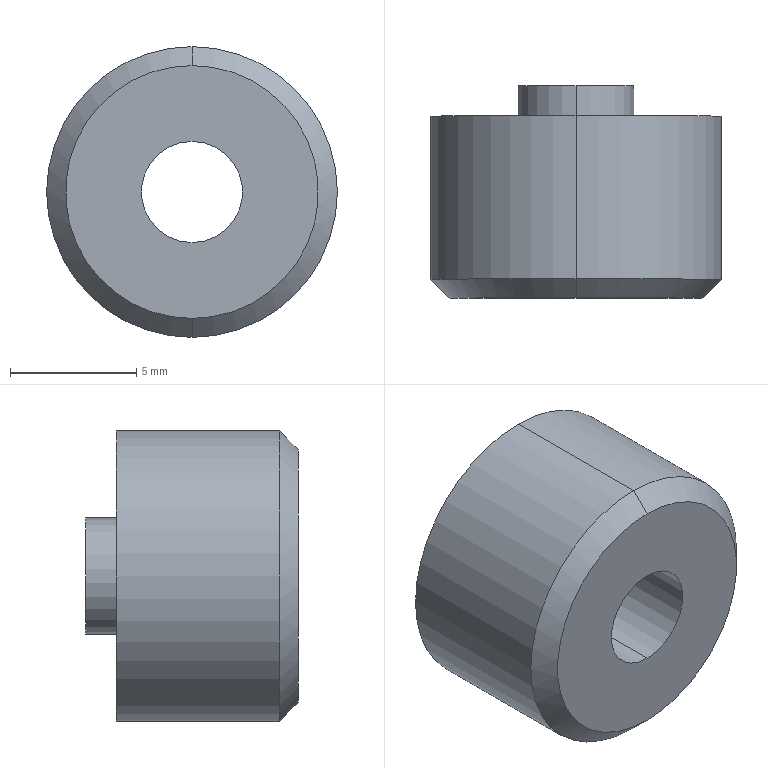Part | STEP file | AC10B-M5_AC3011A AF Drain(10)-1 | 1 solid | 14 faces | box 11.5 x 8.4 x 11.5 mm | volume 268.613 mm3 | cylinder 8 | plane 4 | cone 2 | commonest cylinder face diameters 4 x2 4.6 x2 10 x2 11.5 x2
STEP:
#1=CARTESIAN_POINT('',(0.,0.,0.));
#2=DIRECTION('',(0.,0.,1.));
#3=DIRECTION('',(1.,0.,0.));
#4=AXIS2_PLACEMENT_3D('',#1,#2,#3);
#5=CARTESIAN_POINT('',(0.,-8.4,2.));
#6=VERTEX_POINT('',#5);
#7=CARTESIAN_POINT('',(0.,0.,2.));
#8=VERTEX_POINT('',#7);
#9=CARTESIAN_POINT('',(0.,-8.4,2.));
#10=DIRECTION('',(0.,1.,0.));
#11=VECTOR('',#10,1.);
#12=LINE('',#9,#11);
#13=CARTESIAN_POINT('',(0.,-8.4,0.));
#14=DIRECTION('',(0.,1.,0.));
#15=DIRECTION('',(0.,0.,1.));
#16=AXIS2_PLACEMENT_3D('',#13,#14,#15);
#17=CYLINDRICAL_SURFACE('',#16,2.);
#18=CARTESIAN_POINT('',(6.283,0.));
#19=DIRECTION('',(0.,1.));
#20=VECTOR('',#19,1.);
#21=LINE('',#18,#20);
#22=(GEOMETRIC_REPRESENTATION_CONTEXT(2)PARAMETRIC_REPRESENTATION_CONTEXT()REPRESENTATION_CONTEXT('',''));
#23=DEFINITIONAL_REPRESENTATION('',(#21),#22);
#24=PCURVE('',#17,#23);
#25=CARTESIAN_POINT('',(0.,-8.4,0.));
#26=DIRECTION('',(0.,1.,0.));
#27=DIRECTION('',(0.,0.,1.));
#28=AXIS2_PLACEMENT_3D('',#25,#26,#27);
#29=CYLINDRICAL_SURFACE('',#28,2.);
#30=CARTESIAN_POINT('',(0.,0.));
#31=DIRECTION('',(0.,1.));
#32=VECTOR('',#31,1.);
#33=LINE('',#30,#32);
#34=(GEOMETRIC_REPRESENTATION_CONTEXT(2)PARAMETRIC_REPRESENTATION_CONTEXT()REPRESENTATION_CONTEXT('',''));
#35=DEFINITIONAL_REPRESENTATION('',(#33),#34);
#36=PCURVE('',#29,#35);
#37=SURFACE_CURVE('',#12,(#24,#36),.PCURVE_S1.);
#38=EDGE_CURVE('',#6,#8,#37,.T.);
#39=ORIENTED_EDGE('',*,*,#38,.T.);
#40=CARTESIAN_POINT('',(0.,0.,-2.));
#41=VERTEX_POINT('',#40);
#42=CARTESIAN_POINT('',(0.,0.,0.));
#43=DIRECTION('',(0.,1.,0.));
#44=DIRECTION('',(0.,0.,1.));
#45=AXIS2_PLACEMENT_3D('',#42,#43,#44);
#46=CIRCLE('',#45,2.);
#47=CARTESIAN_POINT('',(0.,8.4));
#48=DIRECTION('',(1.,0.));
#49=VECTOR('',#48,1.);
#50=LINE('',#47,#49);
#51=(GEOMETRIC_REPRESENTATION_CONTEXT(2)PARAMETRIC_REPRESENTATION_CONTEXT()REPRESENTATION_CONTEXT('',''));
#52=DEFINITIONAL_REPRESENTATION('',(#50),#51);
#53=PCURVE('',#17,#52);
#54=CARTESIAN_POINT('',(0.,0.,0.));
#55=DIRECTION('',(0.,1.,0.));
#56=DIRECTION('',(0.,0.,1.));
#57=AXIS2_PLACEMENT_3D('',#54,#55,#56);
#58=PLANE('',#57);
#59=CARTESIAN_POINT('',(0.,0.));
#60=DIRECTION('',(1.,0.));
#61=AXIS2_PLACEMENT_2D('',#59,#60);
#62=CIRCLE('',#61,2.);
#63=(GEOMETRIC_REPRESENTATION_CONTEXT(2)PARAMETRIC_REPRESENTATION_CONTEXT()REPRESENTATION_CONTEXT('',''));
#64=DEFINITIONAL_REPRESENTATION('',(#62),#63);
#65=PCURVE('',#58,#64);
#66=SURFACE_CURVE('',#46,(#53,#65),.PCURVE_S1.);
#67=EDGE_CURVE('',#41,#8,#66,.T.);
#68=ORIENTED_EDGE('',*,*,#67,.F.);
#69=CARTESIAN_POINT('',(0.,-8.4,-2.));
#70=VERTEX_POINT('',#69);
#71=CARTESIAN_POINT('',(0.,-8.4,-2.));
#72=DIRECTION('',(0.,1.,0.));
#73=VECTOR('',#72,1.);
#74=LINE('',#71,#73);
#75=CARTESIAN_POINT('',(3.142,0.));
#76=DIRECTION('',(0.,1.));
#77=VECTOR('',#76,1.);
#78=LINE('',#75,#77);
#79=(GEOMETRIC_REPRESENTATION_CONTEXT(2)PARAMETRIC_REPRESENTATION_CONTEXT()REPRESENTATION_CONTEXT('',''));
#80=DEFINITIONAL_REPRESENTATION('',(#78),#79);
#81=PCURVE('',#17,#80);
#82=CARTESIAN_POINT('',(3.142,0.));
#83=DIRECTION('',(0.,1.));
#84=VECTOR('',#83,1.);
#85=LINE('',#82,#84);
#86=(GEOMETRIC_REPRESENTATION_CONTEXT(2)PARAMETRIC_REPRESENTATION_CONTEXT()REPRESENTATION_CONTEXT('',''));
#87=DEFINITIONAL_REPRESENTATION('',(#85),#86);
#88=PCURVE('',#29,#87);
#89=SURFACE_CURVE('',#74,(#81,#88),.PCURVE_S1.);
#90=EDGE_CURVE('',#70,#41,#89,.T.);
#91=ORIENTED_EDGE('',*,*,#90,.F.);
#92=CARTESIAN_POINT('',(0.,-8.4,0.));
#93=DIRECTION('',(0.,1.,0.));
#94=DIRECTION('',(0.,0.,1.));
#95=AXIS2_PLACEMENT_3D('',#92,#93,#94);
#96=CIRCLE('',#95,2.);
#97=CARTESIAN_POINT('',(0.,0.));
#98=DIRECTION('',(1.,0.));
#99=VECTOR('',#98,1.);
#100=LINE('',#97,#99);
#101=(GEOMETRIC_REPRESENTATION_CONTEXT(2)PARAMETRIC_REPRESENTATION_CONTEXT()REPRESENTATION_CONTEXT('',''));
#102=DEFINITIONAL_REPRESENTATION('',(#100),#101);
#103=PCURVE('',#17,#102);
#104=CARTESIAN_POINT('',(0.,-8.4,0.));
#105=DIRECTION('',(0.,-1.,0.));
#106=DIRECTION('',(0.,0.,-1.));
#107=AXIS2_PLACEMENT_3D('',#104,#105,#106);
#108=PLANE('',#107);
#109=CARTESIAN_POINT('',(-2.,0.));
#110=CARTESIAN_POINT('',(-2.,3.464));
#111=CARTESIAN_POINT('',(1.,1.732));
#112=CARTESIAN_POINT('',(4.,0.));
#113=CARTESIAN_POINT('',(1.,-1.732));
#114=CARTESIAN_POINT('',(-2.,-3.464));
#115=CARTESIAN_POINT('',(-2.,0.));
#116=(BOUNDED_CURVE()B_SPLINE_CURVE(2,(#109,#110,#111,#112,#113,#114,#115),.UNSPECIFIED.,.T.,.F.)B_SPLINE_CURVE_WITH_KNOTS((1,2,2,2,2,1),(-2.094,0.,2.094,4.189,6.283,8.378),.UNSPECIFIED.)CURVE()GEOMETRIC_REPRESENTATION_ITEM()RATIONAL_B_SPLINE_CURVE((1.,0.5,1.,0.5,1.,0.5,1.))REPRESENTATION_ITEM(''));
#117=(GEOMETRIC_REPRESENTATION_CONTEXT(2)PARAMETRIC_REPRESENTATION_CONTEXT()REPRESENTATION_CONTEXT('',''));
#118=DEFINITIONAL_REPRESENTATION('',(#116),#117);
#119=PCURVE('',#108,#118);
#120=SURFACE_CURVE('',#96,(#103,#119),.PCURVE_S1.);
#121=EDGE_CURVE('',#70,#6,#120,.T.);
#122=ORIENTED_EDGE('',*,*,#121,.T.);
#123=EDGE_LOOP('',(#39,#68,#91,#122));
#124=FACE_BOUND('',#123,.F.);
#125=ADVANCED_FACE('',(#124),#17,.F.);
#126=CARTESIAN_POINT('',(0.,-8.4,-5.));
#127=VERTEX_POINT('',#126);
#128=CARTESIAN_POINT('',(0.,-8.4,5.));
#129=VERTEX_POINT('',#128);
#130=CARTESIAN_POINT('',(0.,-8.4,0.));
#131=DIRECTION('',(0.,-1.,0.));
#132=DIRECTION('',(0.,0.,-1.));
#133=AXIS2_PLACEMENT_3D('',#130,#131,#132);
#134=CIRCLE('',#133,5.);
#135=CARTESIAN_POINT('',(0.,-8.4,0.));
#136=DIRECTION('',(0.,1.,0.));
#137=DIRECTION('',(0.,0.,1.));
#138=AXIS2_PLACEMENT_3D('',#135,#136,#137);
#139=CONICAL_SURFACE('',#138,5.,0.7854);
#140=CARTESIAN_POINT('',(3.142,0.));
#141=DIRECTION('',(-1.,0.));
#142=VECTOR('',#141,1.);
#143=LINE('',#140,#142);
#144=(GEOMETRIC_REPRESENTATION_CONTEXT(2)PARAMETRIC_REPRESENTATION_CONTEXT()REPRESENTATION_CONTEXT('',''));
#145=DEFINITIONAL_REPRESENTATION('',(#143),#144);
#146=PCURVE('',#139,#145);
#147=CARTESIAN_POINT('',(0.,0.));
#148=DIRECTION('',(1.,0.));
#149=AXIS2_PLACEMENT_2D('',#147,#148);
#150=CIRCLE('',#149,5.);
#151=(GEOMETRIC_REPRESENTATION_CONTEXT(2)PARAMETRIC_REPRESENTATION_CONTEXT()REPRESENTATION_CONTEXT('',''));
#152=DEFINITIONAL_REPRESENTATION('',(#150),#151);
#153=PCURVE('',#108,#152);
#154=SURFACE_CURVE('',#134,(#146,#153),.PCURVE_S1.);
#155=EDGE_CURVE('',#127,#129,#154,.T.);
#156=ORIENTED_EDGE('',*,*,#155,.F.);
#157=CARTESIAN_POINT('',(0.,-7.65,-5.75));
#158=VERTEX_POINT('',#157);
#159=CARTESIAN_POINT('',(0.,-8.4,-5.));
#160=DIRECTION('',(0.,0.7071,-0.7071));
#161=VECTOR('',#160,1.);
#162=LINE('',#159,#161);
#163=CARTESIAN_POINT('',(3.142,0.));
#164=DIRECTION('',(0.,1.));
#165=VECTOR('',#164,1.);
#166=LINE('',#163,#165);
#167=(GEOMETRIC_REPRESENTATION_CONTEXT(2)PARAMETRIC_REPRESENTATION_CONTEXT()REPRESENTATION_CONTEXT('',''));
#168=DEFINITIONAL_REPRESENTATION('',(#166),#167);
#169=PCURVE('',#139,#168);
#170=CARTESIAN_POINT('',(0.,-8.4,0.));
#171=DIRECTION('',(0.,1.,0.));
#172=DIRECTION('',(0.,0.,1.));
#173=AXIS2_PLACEMENT_3D('',#170,#171,#172);
#174=CONICAL_SURFACE('',#173,5.,0.7854);
#175=CARTESIAN_POINT('',(3.142,0.));
#176=DIRECTION('',(0.,1.));
#177=VECTOR('',#176,1.);
#178=LINE('',#175,#177);
#179=(GEOMETRIC_REPRESENTATION_CONTEXT(2)PARAMETRIC_REPRESENTATION_CONTEXT()REPRESENTATION_CONTEXT('',''));
#180=DEFINITIONAL_REPRESENTATION('',(#178),#179);
#181=PCURVE('',#174,#180);
#182=SURFACE_CURVE('',#162,(#169,#181),.PCURVE_S1.);
#183=EDGE_CURVE('',#127,#158,#182,.T.);
#184=ORIENTED_EDGE('',*,*,#183,.T.);
#185=CARTESIAN_POINT('',(0.,-7.65,5.75));
#186=VERTEX_POINT('',#185);
#187=CARTESIAN_POINT('',(0.,-7.65,0.));
#188=DIRECTION('',(0.,1.,0.));
#189=DIRECTION('',(0.,0.,-1.));
#190=AXIS2_PLACEMENT_3D('',#187,#188,#189);
#191=CIRCLE('',#190,5.75);
#192=CARTESIAN_POINT('',(-3.142,0.75));
#193=DIRECTION('',(1.,0.));
#194=VECTOR('',#193,1.);
#195=LINE('',#192,#194);
#196=(GEOMETRIC_REPRESENTATION_CONTEXT(2)PARAMETRIC_REPRESENTATION_CONTEXT()REPRESENTATION_CONTEXT('',''));
#197=DEFINITIONAL_REPRESENTATION('',(#195),#196);
#198=PCURVE('',#139,#197);
#199=CARTESIAN_POINT('',(0.,-8.4,0.));
#200=DIRECTION('',(0.,1.,0.));
#201=DIRECTION('',(0.,0.,1.));
#202=AXIS2_PLACEMENT_3D('',#199,#200,#201);
#203=CYLINDRICAL_SURFACE('',#202,5.75);
#204=CARTESIAN_POINT('',(-3.142,0.75));
#205=DIRECTION('',(1.,0.));
#206=VECTOR('',#205,1.);
#207=LINE('',#204,#206);
#208=(GEOMETRIC_REPRESENTATION_CONTEXT(2)PARAMETRIC_REPRESENTATION_CONTEXT()REPRESENTATION_CONTEXT('',''));
#209=DEFINITIONAL_REPRESENTATION('',(#207),#208);
#210=PCURVE('',#203,#209);
#211=SURFACE_CURVE('',#191,(#198,#210),.PCURVE_S1.);
#212=EDGE_CURVE('',#186,#158,#211,.T.);
#213=ORIENTED_EDGE('',*,*,#212,.F.);
#214=CARTESIAN_POINT('',(0.,-8.4,5.));
#215=DIRECTION('',(0.,0.7071,0.7071));
#216=VECTOR('',#215,1.);
#217=LINE('',#214,#216);
#218=CARTESIAN_POINT('',(0.,0.));
#219=DIRECTION('',(0.,1.));
#220=VECTOR('',#219,1.);
#221=LINE('',#218,#220);
#222=(GEOMETRIC_REPRESENTATION_CONTEXT(2)PARAMETRIC_REPRESENTATION_CONTEXT()REPRESENTATION_CONTEXT('',''));
#223=DEFINITIONAL_REPRESENTATION('',(#221),#222);
#224=PCURVE('',#139,#223);
#225=CARTESIAN_POINT('',(6.283,0.));
#226=DIRECTION('',(0.,1.));
#227=VECTOR('',#226,1.);
#228=LINE('',#225,#227);
#229=(GEOMETRIC_REPRESENTATION_CONTEXT(2)PARAMETRIC_REPRESENTATION_CONTEXT()REPRESENTATION_CONTEXT('',''));
#230=DEFINITIONAL_REPRESENTATION('',(#228),#229);
#231=PCURVE('',#174,#230);
#232=SURFACE_CURVE('',#217,(#224,#231),.PCURVE_S1.);
#233=EDGE_CURVE('',#129,#186,#232,.T.);
#234=ORIENTED_EDGE('',*,*,#233,.F.);
#235=EDGE_LOOP('',(#156,#184,#213,#234));
#236=FACE_BOUND('',#235,.T.);
#237=ADVANCED_FACE('',(#236),#139,.T.);
#238=CARTESIAN_POINT('',(0.,-7.4,2.3));
#239=VERTEX_POINT('',#238);
#240=CARTESIAN_POINT('',(0.,-7.4,-2.3));
#241=VERTEX_POINT('',#240);
#242=CARTESIAN_POINT('',(0.,-7.4,0.));
#243=DIRECTION('',(0.,1.,0.));
#244=DIRECTION('',(0.,0.,-1.));
#245=AXIS2_PLACEMENT_3D('',#242,#243,#244);
#246=CIRCLE('',#245,2.3);
#247=CARTESIAN_POINT('',(0.,-1.2,0.));
#248=DIRECTION('',(0.,1.,0.));
#249=DIRECTION('',(0.,0.,1.));
#250=AXIS2_PLACEMENT_3D('',#247,#248,#249);
#251=CYLINDRICAL_SURFACE('',#250,2.3);
#252=CARTESIAN_POINT('',(-3.142,-6.2));
#253=DIRECTION('',(1.,0.));
#254=VECTOR('',#253,1.);
#255=LINE('',#252,#254);
#256=(GEOMETRIC_REPRESENTATION_CONTEXT(2)PARAMETRIC_REPRESENTATION_CONTEXT()REPRESENTATION_CONTEXT('',''));
#257=DEFINITIONAL_REPRESENTATION('',(#255),#256);
#258=PCURVE('',#251,#257);
#259=CARTESIAN_POINT('',(0.,-7.4,0.));
#260=DIRECTION('',(0.,-1.,0.));
#261=DIRECTION('',(0.,0.,-1.));
#262=AXIS2_PLACEMENT_3D('',#259,#260,#261);
#263=PLANE('',#262);
#264=CARTESIAN_POINT('',(2.3,0.));
#265=CARTESIAN_POINT('',(2.3,-3.984));
#266=CARTESIAN_POINT('',(-1.15,-1.992));
#267=CARTESIAN_POINT('',(-4.6,0.));
#268=CARTESIAN_POINT('',(-1.15,1.992));
#269=CARTESIAN_POINT('',(2.3,3.984));
#270=CARTESIAN_POINT('',(2.3,0.));
#271=(BOUNDED_CURVE()B_SPLINE_CURVE(2,(#264,#265,#266,#267,#268,#269,#270),.UNSPECIFIED.,.T.,.F.)B_SPLINE_CURVE_WITH_KNOTS((1,2,2,2,2,1),(-2.094,0.,2.094,4.189,6.283,8.378),.UNSPECIFIED.)CURVE()GEOMETRIC_REPRESENTATION_ITEM()RATIONAL_B_SPLINE_CURVE((1.,0.5,1.,0.5,1.,0.5,1.))REPRESENTATION_ITEM(''));
#272=(GEOMETRIC_REPRESENTATION_CONTEXT(2)PARAMETRIC_REPRESENTATION_CONTEXT()REPRESENTATION_CONTEXT('',''));
#273=DEFINITIONAL_REPRESENTATION('',(#271),#272);
#274=PCURVE('',#263,#273);
#275=SURFACE_CURVE('',#246,(#258,#274),.PCURVE_S1.);
#276=EDGE_CURVE('',#239,#241,#275,.T.);
#277=ORIENTED_EDGE('',*,*,#276,.T.);
#278=CARTESIAN_POINT('',(0.,0.,-2.3));
#279=VERTEX_POINT('',#278);
#280=CARTESIAN_POINT('',(0.,-1.2,-2.3));
#281=DIRECTION('',(0.,1.,0.));
#282=VECTOR('',#281,1.);
#283=LINE('',#280,#282);
#284=CARTESIAN_POINT('',(3.142,0.));
#285=DIRECTION('',(0.,1.));
#286=VECTOR('',#285,1.);
#287=LINE('',#284,#286);
#288=(GEOMETRIC_REPRESENTATION_CONTEXT(2)PARAMETRIC_REPRESENTATION_CONTEXT()REPRESENTATION_CONTEXT('',''));
#289=DEFINITIONAL_REPRESENTATION('',(#287),#288);
#290=PCURVE('',#251,#289);
#291=CARTESIAN_POINT('',(0.,-1.2,0.));
#292=DIRECTION('',(0.,1.,0.));
#293=DIRECTION('',(0.,0.,1.));
#294=AXIS2_PLACEMENT_3D('',#291,#292,#293);
#295=CYLINDRICAL_SURFACE('',#294,2.3);
#296=CARTESIAN_POINT('',(3.142,0.));
#297=DIRECTION('',(0.,1.));
#298=VECTOR('',#297,1.);
#299=LINE('',#296,#298);
#300=(GEOMETRIC_REPRESENTATION_CONTEXT(2)PARAMETRIC_REPRESENTATION_CONTEXT()REPRESENTATION_CONTEXT('',''));
#301=DEFINITIONAL_REPRESENTATION('',(#299),#300);
#302=PCURVE('',#295,#301);
#303=SURFACE_CURVE('',#283,(#290,#302),.PCURVE_S1.);
#304=EDGE_CURVE('',#241,#279,#303,.T.);
#305=ORIENTED_EDGE('',*,*,#304,.T.);
#306=CARTESIAN_POINT('',(0.,0.,2.3));
#307=VERTEX_POINT('',#306);
#308=CARTESIAN_POINT('',(0.,0.,0.));
#309=DIRECTION('',(0.,1.,0.));
#310=DIRECTION('',(0.,0.,1.));
#311=AXIS2_PLACEMENT_3D('',#308,#309,#310);
#312=CIRCLE('',#311,2.3);
#313=CARTESIAN_POINT('',(0.,1.2));
#314=DIRECTION('',(1.,0.));
#315=VECTOR('',#314,1.);
#316=LINE('',#313,#315);
#317=(GEOMETRIC_REPRESENTATION_CONTEXT(2)PARAMETRIC_REPRESENTATION_CONTEXT()REPRESENTATION_CONTEXT('',''));
#318=DEFINITIONAL_REPRESENTATION('',(#316),#317);
#319=PCURVE('',#251,#318);
#320=CARTESIAN_POINT('',(0.,0.));
#321=DIRECTION('',(1.,0.));
#322=AXIS2_PLACEMENT_2D('',#320,#321);
#323=CIRCLE('',#322,2.3);
#324=(GEOMETRIC_REPRESENTATION_CONTEXT(2)PARAMETRIC_REPRESENTATION_CONTEXT()REPRESENTATION_CONTEXT('',''));
#325=DEFINITIONAL_REPRESENTATION('',(#323),#324);
#326=PCURVE('',#58,#325);
#327=SURFACE_CURVE('',#312,(#319,#326),.PCURVE_S1.);
#328=EDGE_CURVE('',#307,#279,#327,.T.);
#329=ORIENTED_EDGE('',*,*,#328,.F.);
#330=CARTESIAN_POINT('',(0.,-1.2,2.3));
#331=DIRECTION('',(0.,1.,0.));
#332=VECTOR('',#331,1.);
#333=LINE('',#330,#332);
#334=CARTESIAN_POINT('',(0.,0.));
#335=DIRECTION('',(0.,1.));
#336=VECTOR('',#335,1.);
#337=LINE('',#334,#336);
#338=(GEOMETRIC_REPRESENTATION_CONTEXT(2)PARAMETRIC_REPRESENTATION_CONTEXT()REPRESENTATION_CONTEXT('',''));
#339=DEFINITIONAL_REPRESENTATION('',(#337),#338);
#340=PCURVE('',#251,#339);
#341=CARTESIAN_POINT('',(6.283,0.));
#342=DIRECTION('',(0.,1.));
#343=VECTOR('',#342,1.);
#344=LINE('',#341,#343);
#345=(GEOMETRIC_REPRESENTATION_CONTEXT(2)PARAMETRIC_REPRESENTATION_CONTEXT()REPRESENTATION_CONTEXT('',''));
#346=DEFINITIONAL_REPRESENTATION('',(#344),#345);
#347=PCURVE('',#295,#346);
#348=SURFACE_CURVE('',#333,(#340,#347),.PCURVE_S1.);
#349=EDGE_CURVE('',#239,#307,#348,.T.);
#350=ORIENTED_EDGE('',*,*,#349,.F.);
#351=EDGE_LOOP('',(#277,#305,#329,#350));
#352=FACE_BOUND('',#351,.T.);
#353=ADVANCED_FACE('',(#352),#251,.T.);
#354=CARTESIAN_POINT('',(0.,-7.4,5.));
#355=VERTEX_POINT('',#354);
#356=CARTESIAN_POINT('',(0.,-1.2,5.));
#357=VERTEX_POINT('',#356);
#358=CARTESIAN_POINT('',(0.,-22.542,5.));
#359=DIRECTION('',(0.,1.,0.));
#360=VECTOR('',#359,1.);
#361=LINE('',#358,#360);
#362=CARTESIAN_POINT('',(0.,-22.542,0.));
#363=DIRECTION('',(0.,1.,0.));
#364=DIRECTION('',(0.,0.,1.));
#365=AXIS2_PLACEMENT_3D('',#362,#363,#364);
#366=CYLINDRICAL_SURFACE('',#365,5.);
#367=CARTESIAN_POINT('',(6.283,0.));
#368=DIRECTION('',(0.,1.));
#369=VECTOR('',#368,1.);
#370=LINE('',#367,#369);
#371=(GEOMETRIC_REPRESENTATION_CONTEXT(2)PARAMETRIC_REPRESENTATION_CONTEXT()REPRESENTATION_CONTEXT('',''));
#372=DEFINITIONAL_REPRESENTATION('',(#370),#371);
#373=PCURVE('',#366,#372);
#374=CARTESIAN_POINT('',(0.,-22.542,0.));
#375=DIRECTION('',(0.,1.,0.));
#376=DIRECTION('',(0.,0.,1.));
#377=AXIS2_PLACEMENT_3D('',#374,#375,#376);
#378=CYLINDRICAL_SURFACE('',#377,5.);
#379=CARTESIAN_POINT('',(0.,0.));
#380=DIRECTION('',(0.,1.));
#381=VECTOR('',#380,1.);
#382=LINE('',#379,#381);
#383=(GEOMETRIC_REPRESENTATION_CONTEXT(2)PARAMETRIC_REPRESENTATION_CONTEXT()REPRESENTATION_CONTEXT('',''));
#384=DEFINITIONAL_REPRESENTATION('',(#382),#383);
#385=PCURVE('',#378,#384);
#386=SURFACE_CURVE('',#361,(#373,#385),.PCURVE_S1.);
#387=EDGE_CURVE('',#355,#357,#386,.T.);
#388=ORIENTED_EDGE('',*,*,#387,.T.);
#389=CARTESIAN_POINT('',(0.,-1.2,-5.));
#390=VERTEX_POINT('',#389);
#391=CARTESIAN_POINT('',(0.,-1.2,0.));
#392=DIRECTION('',(0.,1.,0.));
#393=DIRECTION('',(0.,0.,1.));
#394=AXIS2_PLACEMENT_3D('',#391,#392,#393);
#395=CIRCLE('',#394,5.);
#396=CARTESIAN_POINT('',(0.,21.342));
#397=DIRECTION('',(1.,0.));
#398=VECTOR('',#397,1.);
#399=LINE('',#396,#398);
#400=(GEOMETRIC_REPRESENTATION_CONTEXT(2)PARAMETRIC_REPRESENTATION_CONTEXT()REPRESENTATION_CONTEXT('',''));
#401=DEFINITIONAL_REPRESENTATION('',(#399),#400);
#402=PCURVE('',#366,#401);
#403=CARTESIAN_POINT('',(0.,-1.2,0.));
#404=DIRECTION('',(0.,-1.,0.));
#405=DIRECTION('',(0.,0.,-1.));
#406=AXIS2_PLACEMENT_3D('',#403,#404,#405);
#407=PLANE('',#406);
#408=CARTESIAN_POINT('',(-5.,0.));
#409=CARTESIAN_POINT('',(-5.,8.66));
#410=CARTESIAN_POINT('',(2.5,4.33));
#411=CARTESIAN_POINT('',(10.,0.));
#412=CARTESIAN_POINT('',(2.5,-4.33));
#413=CARTESIAN_POINT('',(-5.,-8.66));
#414=CARTESIAN_POINT('',(-5.,0.));
#415=(BOUNDED_CURVE()B_SPLINE_CURVE(2,(#408,#409,#410,#411,#412,#413,#414),.UNSPECIFIED.,.T.,.F.)B_SPLINE_CURVE_WITH_KNOTS((1,2,2,2,2,1),(-2.094,0.,2.094,4.189,6.283,8.378),.UNSPECIFIED.)CURVE()GEOMETRIC_REPRESENTATION_ITEM()RATIONAL_B_SPLINE_CURVE((1.,0.5,1.,0.5,1.,0.5,1.))REPRESENTATION_ITEM(''));
#416=(GEOMETRIC_REPRESENTATION_CONTEXT(2)PARAMETRIC_REPRESENTATION_CONTEXT()REPRESENTATION_CONTEXT('',''));
#417=DEFINITIONAL_REPRESENTATION('',(#415),#416);
#418=PCURVE('',#407,#417);
#419=SURFACE_CURVE('',#395,(#402,#418),.PCURVE_S1.);
#420=EDGE_CURVE('',#390,#357,#419,.T.);
#421=ORIENTED_EDGE('',*,*,#420,.F.);
#422=CARTESIAN_POINT('',(0.,-7.4,-5.));
#423=VERTEX_POINT('',#422);
#424=CARTESIAN_POINT('',(0.,-22.542,-5.));
#425=DIRECTION('',(0.,1.,0.));
#426=VECTOR('',#425,1.);
#427=LINE('',#424,#426);
#428=CARTESIAN_POINT('',(3.142,0.));
#429=DIRECTION('',(0.,1.));
#430=VECTOR('',#429,1.);
#431=LINE('',#428,#430);
#432=(GEOMETRIC_REPRESENTATION_CONTEXT(2)PARAMETRIC_REPRESENTATION_CONTEXT()REPRESENTATION_CONTEXT('',''));
#433=DEFINITIONAL_REPRESENTATION('',(#431),#432);
#434=PCURVE('',#366,#433);
#435=CARTESIAN_POINT('',(3.142,0.));
#436=DIRECTION('',(0.,1.));
#437=VECTOR('',#436,1.);
#438=LINE('',#435,#437);
#439=(GEOMETRIC_REPRESENTATION_CONTEXT(2)PARAMETRIC_REPRESENTATION_CONTEXT()REPRESENTATION_CONTEXT('',''));
#440=DEFINITIONAL_REPRESENTATION('',(#438),#439);
#441=PCURVE('',#378,#440);
#442=SURFACE_CURVE('',#427,(#434,#441),.PCURVE_S1.);
#443=EDGE_CURVE('',#423,#390,#442,.T.);
#444=ORIENTED_EDGE('',*,*,#443,.F.);
#445=CARTESIAN_POINT('',(0.,-7.4,0.));
#446=DIRECTION('',(0.,1.,0.));
#447=DIRECTION('',(0.,0.,-1.));
#448=AXIS2_PLACEMENT_3D('',#445,#446,#447);
#449=CIRCLE('',#448,5.);
#450=CARTESIAN_POINT('',(3.142,15.142));
#451=DIRECTION('',(1.,0.));
#452=VECTOR('',#451,1.);
#453=LINE('',#450,#452);
#454=(GEOMETRIC_REPRESENTATION_CONTEXT(2)PARAMETRIC_REPRESENTATION_CONTEXT()REPRESENTATION_CONTEXT('',''));
#455=DEFINITIONAL_REPRESENTATION('',(#453),#454);
#456=PCURVE('',#366,#455);
#457=CARTESIAN_POINT('',(5.,0.));
#458=CARTESIAN_POINT('',(5.,-8.66));
#459=CARTESIAN_POINT('',(-2.5,-4.33));
#460=CARTESIAN_POINT('',(-10.,0.));
#461=CARTESIAN_POINT('',(-2.5,4.33));
#462=CARTESIAN_POINT('',(5.,8.66));
#463=CARTESIAN_POINT('',(5.,0.));
#464=(BOUNDED_CURVE()B_SPLINE_CURVE(2,(#457,#458,#459,#460,#461,#462,#463),.UNSPECIFIED.,.T.,.F.)B_SPLINE_CURVE_WITH_KNOTS((1,2,2,2,2,1),(-2.094,0.,2.094,4.189,6.283,8.378),.UNSPECIFIED.)CURVE()GEOMETRIC_REPRESENTATION_ITEM()RATIONAL_B_SPLINE_CURVE((1.,0.5,1.,0.5,1.,0.5,1.))REPRESENTATION_ITEM(''));
#465=(GEOMETRIC_REPRESENTATION_CONTEXT(2)PARAMETRIC_REPRESENTATION_CONTEXT()REPRESENTATION_CONTEXT('',''));
#466=DEFINITIONAL_REPRESENTATION('',(#464),#465);
#467=PCURVE('',#263,#466);
#468=SURFACE_CURVE('',#449,(#456,#467),.PCURVE_S1.);
#469=EDGE_CURVE('',#423,#355,#468,.T.);
#470=ORIENTED_EDGE('',*,*,#469,.T.);
#471=EDGE_LOOP('',(#388,#421,#444,#470));
#472=FACE_BOUND('',#471,.F.);
#473=ADVANCED_FACE('',(#472),#366,.F.);
#474=ORIENTED_EDGE('',*,*,#212,.T.);
#475=CARTESIAN_POINT('',(0.,-1.2,-5.75));
#476=VERTEX_POINT('',#475);
#477=CARTESIAN_POINT('',(0.,-8.4,-5.75));
#478=DIRECTION('',(0.,1.,0.));
#479=VECTOR('',#478,1.);
#480=LINE('',#477,#479);
#481=CARTESIAN_POINT('',(3.142,0.));
#482=DIRECTION('',(0.,1.));
#483=VECTOR('',#482,1.);
#484=LINE('',#481,#483);
#485=(GEOMETRIC_REPRESENTATION_CONTEXT(2)PARAMETRIC_REPRESENTATION_CONTEXT()REPRESENTATION_CONTEXT('',''));
#486=DEFINITIONAL_REPRESENTATION('',(#484),#485);
#487=PCURVE('',#203,#486);
#488=CARTESIAN_POINT('',(0.,-8.4,0.));
#489=DIRECTION('',(0.,1.,0.));
#490=DIRECTION('',(0.,0.,1.));
#491=AXIS2_PLACEMENT_3D('',#488,#489,#490);
#492=CYLINDRICAL_SURFACE('',#491,5.75);
#493=CARTESIAN_POINT('',(3.142,0.));
#494=DIRECTION('',(0.,1.));
#495=VECTOR('',#494,1.);
#496=LINE('',#493,#495);
#497=(GEOMETRIC_REPRESENTATION_CONTEXT(2)PARAMETRIC_REPRESENTATION_CONTEXT()REPRESENTATION_CONTEXT('',''));
#498=DEFINITIONAL_REPRESENTATION('',(#496),#497);
#499=PCURVE('',#492,#498);
#500=SURFACE_CURVE('',#480,(#487,#499),.PCURVE_S1.);
#501=EDGE_CURVE('',#158,#476,#500,.T.);
#502=ORIENTED_EDGE('',*,*,#501,.T.);
#503=CARTESIAN_POINT('',(0.,-1.2,5.75));
#504=VERTEX_POINT('',#503);
#505=CARTESIAN_POINT('',(0.,-1.2,0.));
#506=DIRECTION('',(0.,-1.,0.));
#507=DIRECTION('',(0.,0.,-1.));
#508=AXIS2_PLACEMENT_3D('',#505,#506,#507);
#509=CIRCLE('',#508,5.75);
#510=CARTESIAN_POINT('',(3.142,7.2));
#511=DIRECTION('',(-1.,0.));
#512=VECTOR('',#511,1.);
#513=LINE('',#510,#512);
#514=(GEOMETRIC_REPRESENTATION_CONTEXT(2)PARAMETRIC_REPRESENTATION_CONTEXT()REPRESENTATION_CONTEXT('',''));
#515=DEFINITIONAL_REPRESENTATION('',(#513),#514);
#516=PCURVE('',#203,#515);
#517=CARTESIAN_POINT('',(0.,0.));
#518=DIRECTION('',(1.,0.));
#519=AXIS2_PLACEMENT_2D('',#517,#518);
#520=CIRCLE('',#519,5.75);
#521=(GEOMETRIC_REPRESENTATION_CONTEXT(2)PARAMETRIC_REPRESENTATION_CONTEXT()REPRESENTATION_CONTEXT('',''));
#522=DEFINITIONAL_REPRESENTATION('',(#520),#521);
#523=PCURVE('',#407,#522);
#524=SURFACE_CURVE('',#509,(#516,#523),.PCURVE_S1.);
#525=EDGE_CURVE('',#476,#504,#524,.T.);
#526=ORIENTED_EDGE('',*,*,#525,.T.);
#527=CARTESIAN_POINT('',(0.,-8.4,5.75));
#528=DIRECTION('',(0.,1.,0.));
#529=VECTOR('',#528,1.);
#530=LINE('',#527,#529);
#531=CARTESIAN_POINT('',(0.,0.));
#532=DIRECTION('',(0.,1.));
#533=VECTOR('',#532,1.);
#534=LINE('',#531,#533);
#535=(GEOMETRIC_REPRESENTATION_CONTEXT(2)PARAMETRIC_REPRESENTATION_CONTEXT()REPRESENTATION_CONTEXT('',''));
#536=DEFINITIONAL_REPRESENTATION('',(#534),#535);
#537=PCURVE('',#203,#536);
#538=CARTESIAN_POINT('',(6.283,0.));
#539=DIRECTION('',(0.,1.));
#540=VECTOR('',#539,1.);
#541=LINE('',#538,#540);
#542=(GEOMETRIC_REPRESENTATION_CONTEXT(2)PARAMETRIC_REPRESENTATION_CONTEXT()REPRESENTATION_CONTEXT('',''));
#543=DEFINITIONAL_REPRESENTATION('',(#541),#542);
#544=PCURVE('',#492,#543);
#545=SURFACE_CURVE('',#530,(#537,#544),.PCURVE_S1.);
#546=EDGE_CURVE('',#186,#504,#545,.T.);
#547=ORIENTED_EDGE('',*,*,#546,.F.);
#548=EDGE_LOOP('',(#474,#502,#526,#547));
#549=FACE_BOUND('',#548,.T.);
#550=ADVANCED_FACE('',(#549),#203,.T.);
#551=ORIENTED_EDGE('',*,*,#501,.F.);
#552=CARTESIAN_POINT('',(0.,-7.65,0.));
#553=DIRECTION('',(0.,1.,0.));
#554=DIRECTION('',(0.,0.,-1.));
#555=AXIS2_PLACEMENT_3D('',#552,#553,#554);
#556=CIRCLE('',#555,5.75);
#557=CARTESIAN_POINT('',(3.142,0.75));
#558=DIRECTION('',(1.,0.));
#559=VECTOR('',#558,1.);
#560=LINE('',#557,#559);
#561=(GEOMETRIC_REPRESENTATION_CONTEXT(2)PARAMETRIC_REPRESENTATION_CONTEXT()REPRESENTATION_CONTEXT('',''));
#562=DEFINITIONAL_REPRESENTATION('',(#560),#561);
#563=PCURVE('',#492,#562);
#564=CARTESIAN_POINT('',(3.142,0.75));
#565=DIRECTION('',(1.,0.));
#566=VECTOR('',#565,1.);
#567=LINE('',#564,#566);
#568=(GEOMETRIC_REPRESENTATION_CONTEXT(2)PARAMETRIC_REPRESENTATION_CONTEXT()REPRESENTATION_CONTEXT('',''));
#569=DEFINITIONAL_REPRESENTATION('',(#567),#568);
#570=PCURVE('',#174,#569);
#571=SURFACE_CURVE('',#556,(#563,#570),.PCURVE_S1.);
#572=EDGE_CURVE('',#158,#186,#571,.T.);
#573=ORIENTED_EDGE('',*,*,#572,.T.);
#574=ORIENTED_EDGE('',*,*,#546,.T.);
#575=CARTESIAN_POINT('',(0.,-1.2,0.));
#576=DIRECTION('',(0.,-1.,0.));
#577=DIRECTION('',(0.,0.,-1.));
#578=AXIS2_PLACEMENT_3D('',#575,#576,#577);
#579=CIRCLE('',#578,5.75);
#580=CARTESIAN_POINT('',(9.425,7.2));
#581=DIRECTION('',(-1.,0.));
#582=VECTOR('',#581,1.);
#583=LINE('',#580,#582);
#584=(GEOMETRIC_REPRESENTATION_CONTEXT(2)PARAMETRIC_REPRESENTATION_CONTEXT()REPRESENTATION_CONTEXT('',''));
#585=DEFINITIONAL_REPRESENTATION('',(#583),#584);
#586=PCURVE('',#492,#585);
#587=CARTESIAN_POINT('',(0.,0.));
#588=DIRECTION('',(1.,0.));
#589=AXIS2_PLACEMENT_2D('',#587,#588);
#590=CIRCLE('',#589,5.75);
#591=(GEOMETRIC_REPRESENTATION_CONTEXT(2)PARAMETRIC_REPRESENTATION_CONTEXT()REPRESENTATION_CONTEXT('',''));
#592=DEFINITIONAL_REPRESENTATION('',(#590),#591);
#593=PCURVE('',#407,#592);
#594=SURFACE_CURVE('',#579,(#586,#593),.PCURVE_S1.);
#595=EDGE_CURVE('',#504,#476,#594,.T.);
#596=ORIENTED_EDGE('',*,*,#595,.T.);
#597=EDGE_LOOP('',(#551,#573,#574,#596));
#598=FACE_BOUND('',#597,.T.);
#599=ADVANCED_FACE('',(#598),#492,.T.);
#600=CARTESIAN_POINT('',(0.,-8.4,0.));
#601=DIRECTION('',(0.,1.,0.));
#602=DIRECTION('',(0.,0.,1.));
#603=AXIS2_PLACEMENT_3D('',#600,#601,#602);
#604=CIRCLE('',#603,2.);
#605=CARTESIAN_POINT('',(-2.,0.));
#606=CARTESIAN_POINT('',(-2.,3.464));
#607=CARTESIAN_POINT('',(1.,1.732));
#608=CARTESIAN_POINT('',(4.,0.));
#609=CARTESIAN_POINT('',(1.,-1.732));
#610=CARTESIAN_POINT('',(-2.,-3.464));
#611=CARTESIAN_POINT('',(-2.,0.));
#612=(BOUNDED_CURVE()B_SPLINE_CURVE(2,(#605,#606,#607,#608,#609,#610,#611),.UNSPECIFIED.,.T.,.F.)B_SPLINE_CURVE_WITH_KNOTS((1,2,2,2,2,1),(-2.094,0.,2.094,4.189,6.283,8.378),.UNSPECIFIED.)CURVE()GEOMETRIC_REPRESENTATION_ITEM()RATIONAL_B_SPLINE_CURVE((1.,0.5,1.,0.5,1.,0.5,1.))REPRESENTATION_ITEM(''));
#613=(GEOMETRIC_REPRESENTATION_CONTEXT(2)PARAMETRIC_REPRESENTATION_CONTEXT()REPRESENTATION_CONTEXT('',''));
#614=DEFINITIONAL_REPRESENTATION('',(#612),#613);
#615=PCURVE('',#108,#614);
#616=CARTESIAN_POINT('',(0.,0.));
#617=DIRECTION('',(1.,0.));
#618=VECTOR('',#617,1.);
#619=LINE('',#616,#618);
#620=(GEOMETRIC_REPRESENTATION_CONTEXT(2)PARAMETRIC_REPRESENTATION_CONTEXT()REPRESENTATION_CONTEXT('',''));
#621=DEFINITIONAL_REPRESENTATION('',(#619),#620);
#622=PCURVE('',#29,#621);
#623=SURFACE_CURVE('',#604,(#615,#622),.PCURVE_S1.);
#624=EDGE_CURVE('',#6,#70,#623,.T.);
#625=ORIENTED_EDGE('',*,*,#624,.T.);
#626=ORIENTED_EDGE('',*,*,#121,.T.);
#627=EDGE_LOOP('',(#625,#626));
#628=FACE_BOUND('',#627,.T.);
#629=CARTESIAN_POINT('',(0.,-8.4,0.));
#630=DIRECTION('',(0.,-1.,0.));
#631=DIRECTION('',(0.,0.,-1.));
#632=AXIS2_PLACEMENT_3D('',#629,#630,#631);
#633=CIRCLE('',#632,5.);
#634=CARTESIAN_POINT('',(0.,0.));
#635=DIRECTION('',(1.,0.));
#636=AXIS2_PLACEMENT_2D('',#634,#635);
#637=CIRCLE('',#636,5.);
#638=(GEOMETRIC_REPRESENTATION_CONTEXT(2)PARAMETRIC_REPRESENTATION_CONTEXT()REPRESENTATION_CONTEXT('',''));
#639=DEFINITIONAL_REPRESENTATION('',(#637),#638);
#640=PCURVE('',#108,#639);
#641=CARTESIAN_POINT('',(9.425,0.));
#642=DIRECTION('',(-1.,0.));
#643=VECTOR('',#642,1.);
#644=LINE('',#641,#643);
#645=(GEOMETRIC_REPRESENTATION_CONTEXT(2)PARAMETRIC_REPRESENTATION_CONTEXT()REPRESENTATION_CONTEXT('',''));
#646=DEFINITIONAL_REPRESENTATION('',(#644),#645);
#647=PCURVE('',#174,#646);
#648=SURFACE_CURVE('',#633,(#640,#647),.PCURVE_S1.);
#649=EDGE_CURVE('',#129,#127,#648,.T.);
#650=ORIENTED_EDGE('',*,*,#649,.T.);
#651=ORIENTED_EDGE('',*,*,#155,.T.);
#652=EDGE_LOOP('',(#650,#651));
#653=FACE_BOUND('',#652,.T.);
#654=ADVANCED_FACE('',(#628,#653),#108,.T.);
#655=CARTESIAN_POINT('',(0.,-1.2,0.));
#656=DIRECTION('',(0.,1.,0.));
#657=DIRECTION('',(0.,0.,1.));
#658=AXIS2_PLACEMENT_3D('',#655,#656,#657);
#659=CIRCLE('',#658,5.);
#660=CARTESIAN_POINT('',(-5.,0.));
#661=CARTESIAN_POINT('',(-5.,8.66));
#662=CARTESIAN_POINT('',(2.5,4.33));
#663=CARTESIAN_POINT('',(10.,0.));
#664=CARTESIAN_POINT('',(2.5,-4.33));
#665=CARTESIAN_POINT('',(-5.,-8.66));
#666=CARTESIAN_POINT('',(-5.,0.));
#667=(BOUNDED_CURVE()B_SPLINE_CURVE(2,(#660,#661,#662,#663,#664,#665,#666),.UNSPECIFIED.,.T.,.F.)B_SPLINE_CURVE_WITH_KNOTS((1,2,2,2,2,1),(-2.094,0.,2.094,4.189,6.283,8.378),.UNSPECIFIED.)CURVE()GEOMETRIC_REPRESENTATION_ITEM()RATIONAL_B_SPLINE_CURVE((1.,0.5,1.,0.5,1.,0.5,1.))REPRESENTATION_ITEM(''));
#668=(GEOMETRIC_REPRESENTATION_CONTEXT(2)PARAMETRIC_REPRESENTATION_CONTEXT()REPRESENTATION_CONTEXT('',''));
#669=DEFINITIONAL_REPRESENTATION('',(#667),#668);
#670=PCURVE('',#407,#669);
#671=CARTESIAN_POINT('',(0.,21.342));
#672=DIRECTION('',(1.,0.));
#673=VECTOR('',#672,1.);
#674=LINE('',#671,#673);
#675=(GEOMETRIC_REPRESENTATION_CONTEXT(2)PARAMETRIC_REPRESENTATION_CONTEXT()REPRESENTATION_CONTEXT('',''));
#676=DEFINITIONAL_REPRESENTATION('',(#674),#675);
#677=PCURVE('',#378,#676);
#678=SURFACE_CURVE('',#659,(#670,#677),.PCURVE_S1.);
#679=EDGE_CURVE('',#357,#390,#678,.T.);
#680=ORIENTED_EDGE('',*,*,#679,.F.);
#681=ORIENTED_EDGE('',*,*,#420,.F.);
#682=EDGE_LOOP('',(#680,#681));
#683=FACE_BOUND('',#682,.T.);
#684=ORIENTED_EDGE('',*,*,#595,.F.);
#685=ORIENTED_EDGE('',*,*,#525,.F.);
#686=EDGE_LOOP('',(#684,#685));
#687=FACE_BOUND('',#686,.T.);
#688=ADVANCED_FACE('',(#683,#687),#407,.F.);
#689=ORIENTED_EDGE('',*,*,#679,.F.);
#690=ORIENTED_EDGE('',*,*,#387,.F.);
#691=CARTESIAN_POINT('',(0.,-7.4,0.));
#692=DIRECTION('',(0.,1.,0.));
#693=DIRECTION('',(0.,0.,-1.));
#694=AXIS2_PLACEMENT_3D('',#691,#692,#693);
#695=CIRCLE('',#694,5.);
#696=CARTESIAN_POINT('',(-3.142,15.142));
#697=DIRECTION('',(1.,0.));
#698=VECTOR('',#697,1.);
#699=LINE('',#696,#698);
#700=(GEOMETRIC_REPRESENTATION_CONTEXT(2)PARAMETRIC_REPRESENTATION_CONTEXT()REPRESENTATION_CONTEXT('',''));
#701=DEFINITIONAL_REPRESENTATION('',(#699),#700);
#702=PCURVE('',#378,#701);
#703=CARTESIAN_POINT('',(5.,0.));
#704=CARTESIAN_POINT('',(5.,-8.66));
#705=CARTESIAN_POINT('',(-2.5,-4.33));
#706=CARTESIAN_POINT('',(-10.,0.));
#707=CARTESIAN_POINT('',(-2.5,4.33));
#708=CARTESIAN_POINT('',(5.,8.66));
#709=CARTESIAN_POINT('',(5.,0.));
#710=(BOUNDED_CURVE()B_SPLINE_CURVE(2,(#703,#704,#705,#706,#707,#708,#709),.UNSPECIFIED.,.T.,.F.)B_SPLINE_CURVE_WITH_KNOTS((1,2,2,2,2,1),(-2.094,0.,2.094,4.189,6.283,8.378),.UNSPECIFIED.)CURVE()GEOMETRIC_REPRESENTATION_ITEM()RATIONAL_B_SPLINE_CURVE((1.,0.5,1.,0.5,1.,0.5,1.))REPRESENTATION_ITEM(''));
#711=(GEOMETRIC_REPRESENTATION_CONTEXT(2)PARAMETRIC_REPRESENTATION_CONTEXT()REPRESENTATION_CONTEXT('',''));
#712=DEFINITIONAL_REPRESENTATION('',(#710),#711);
#713=PCURVE('',#263,#712);
#714=SURFACE_CURVE('',#695,(#702,#713),.PCURVE_S1.);
#715=EDGE_CURVE('',#355,#423,#714,.T.);
#716=ORIENTED_EDGE('',*,*,#715,.T.);
#717=ORIENTED_EDGE('',*,*,#443,.T.);
#718=EDGE_LOOP('',(#689,#690,#716,#717));
#719=FACE_BOUND('',#718,.F.);
#720=ADVANCED_FACE('',(#719),#378,.F.);
#721=ORIENTED_EDGE('',*,*,#715,.T.);
#722=ORIENTED_EDGE('',*,*,#469,.T.);
#723=EDGE_LOOP('',(#721,#722));
#724=FACE_BOUND('',#723,.T.);
#725=ORIENTED_EDGE('',*,*,#276,.F.);
#726=CARTESIAN_POINT('',(0.,-7.4,0.));
#727=DIRECTION('',(0.,1.,0.));
#728=DIRECTION('',(0.,0.,-1.));
#729=AXIS2_PLACEMENT_3D('',#726,#727,#728);
#730=CIRCLE('',#729,2.3);
#731=CARTESIAN_POINT('',(2.3,0.));
#732=CARTESIAN_POINT('',(2.3,-3.984));
#733=CARTESIAN_POINT('',(-1.15,-1.992));
#734=CARTESIAN_POINT('',(-4.6,0.));
#735=CARTESIAN_POINT('',(-1.15,1.992));
#736=CARTESIAN_POINT('',(2.3,3.984));
#737=CARTESIAN_POINT('',(2.3,0.));
#738=(BOUNDED_CURVE()B_SPLINE_CURVE(2,(#731,#732,#733,#734,#735,#736,#737),.UNSPECIFIED.,.T.,.F.)B_SPLINE_CURVE_WITH_KNOTS((1,2,2,2,2,1),(-2.094,0.,2.094,4.189,6.283,8.378),.UNSPECIFIED.)CURVE()GEOMETRIC_REPRESENTATION_ITEM()RATIONAL_B_SPLINE_CURVE((1.,0.5,1.,0.5,1.,0.5,1.))REPRESENTATION_ITEM(''));
#739=(GEOMETRIC_REPRESENTATION_CONTEXT(2)PARAMETRIC_REPRESENTATION_CONTEXT()REPRESENTATION_CONTEXT('',''));
#740=DEFINITIONAL_REPRESENTATION('',(#738),#739);
#741=PCURVE('',#263,#740);
#742=CARTESIAN_POINT('',(3.142,-6.2));
#743=DIRECTION('',(1.,0.));
#744=VECTOR('',#743,1.);
#745=LINE('',#742,#744);
#746=(GEOMETRIC_REPRESENTATION_CONTEXT(2)PARAMETRIC_REPRESENTATION_CONTEXT()REPRESENTATION_CONTEXT('',''));
#747=DEFINITIONAL_REPRESENTATION('',(#745),#746);
#748=PCURVE('',#295,#747);
#749=SURFACE_CURVE('',#730,(#741,#748),.PCURVE_S1.);
#750=EDGE_CURVE('',#241,#239,#749,.T.);
#751=ORIENTED_EDGE('',*,*,#750,.F.);
#752=EDGE_LOOP('',(#725,#751));
#753=FACE_BOUND('',#752,.T.);
#754=ADVANCED_FACE('',(#724,#753),#263,.F.);
#755=CARTESIAN_POINT('',(0.,0.,0.));
#756=DIRECTION('',(0.,1.,0.));
#757=DIRECTION('',(0.,0.,1.));
#758=AXIS2_PLACEMENT_3D('',#755,#756,#757);
#759=CIRCLE('',#758,2.);
#760=CARTESIAN_POINT('',(0.,0.));
#761=DIRECTION('',(1.,0.));
#762=AXIS2_PLACEMENT_2D('',#760,#761);
#763=CIRCLE('',#762,2.);
#764=(GEOMETRIC_REPRESENTATION_CONTEXT(2)PARAMETRIC_REPRESENTATION_CONTEXT()REPRESENTATION_CONTEXT('',''));
#765=DEFINITIONAL_REPRESENTATION('',(#763),#764);
#766=PCURVE('',#58,#765);
#767=CARTESIAN_POINT('',(0.,8.4));
#768=DIRECTION('',(1.,0.));
#769=VECTOR('',#768,1.);
#770=LINE('',#767,#769);
#771=(GEOMETRIC_REPRESENTATION_CONTEXT(2)PARAMETRIC_REPRESENTATION_CONTEXT()REPRESENTATION_CONTEXT('',''));
#772=DEFINITIONAL_REPRESENTATION('',(#770),#771);
#773=PCURVE('',#29,#772);
#774=SURFACE_CURVE('',#759,(#766,#773),.PCURVE_S1.);
#775=EDGE_CURVE('',#8,#41,#774,.T.);
#776=ORIENTED_EDGE('',*,*,#775,.F.);
#777=ORIENTED_EDGE('',*,*,#67,.F.);
#778=EDGE_LOOP('',(#776,#777));
#779=FACE_BOUND('',#778,.T.);
#780=ORIENTED_EDGE('',*,*,#328,.T.);
#781=CARTESIAN_POINT('',(0.,0.,0.));
#782=DIRECTION('',(0.,1.,0.));
#783=DIRECTION('',(0.,0.,1.));
#784=AXIS2_PLACEMENT_3D('',#781,#782,#783);
#785=CIRCLE('',#784,2.3);
#786=CARTESIAN_POINT('',(0.,0.));
#787=DIRECTION('',(1.,0.));
#788=AXIS2_PLACEMENT_2D('',#786,#787);
#789=CIRCLE('',#788,2.3);
#790=(GEOMETRIC_REPRESENTATION_CONTEXT(2)PARAMETRIC_REPRESENTATION_CONTEXT()REPRESENTATION_CONTEXT('',''));
#791=DEFINITIONAL_REPRESENTATION('',(#789),#790);
#792=PCURVE('',#58,#791);
#793=CARTESIAN_POINT('',(0.,1.2));
#794=DIRECTION('',(1.,0.));
#795=VECTOR('',#794,1.);
#796=LINE('',#793,#795);
#797=(GEOMETRIC_REPRESENTATION_CONTEXT(2)PARAMETRIC_REPRESENTATION_CONTEXT()REPRESENTATION_CONTEXT('',''));
#798=DEFINITIONAL_REPRESENTATION('',(#796),#797);
#799=PCURVE('',#295,#798);
#800=SURFACE_CURVE('',#785,(#792,#799),.PCURVE_S1.);
#801=EDGE_CURVE('',#279,#307,#800,.T.);
#802=ORIENTED_EDGE('',*,*,#801,.T.);
#803=EDGE_LOOP('',(#780,#802));
#804=FACE_BOUND('',#803,.T.);
#805=ADVANCED_FACE('',(#779,#804),#58,.T.);
#806=ORIENTED_EDGE('',*,*,#304,.F.);
#807=ORIENTED_EDGE('',*,*,#750,.T.);
#808=ORIENTED_EDGE('',*,*,#349,.T.);
#809=ORIENTED_EDGE('',*,*,#801,.F.);
#810=EDGE_LOOP('',(#806,#807,#808,#809));
#811=FACE_BOUND('',#810,.T.);
#812=ADVANCED_FACE('',(#811),#295,.T.);
#813=ORIENTED_EDGE('',*,*,#183,.F.);
#814=ORIENTED_EDGE('',*,*,#649,.F.);
#815=ORIENTED_EDGE('',*,*,#233,.T.);
#816=ORIENTED_EDGE('',*,*,#572,.F.);
#817=EDGE_LOOP('',(#813,#814,#815,#816));
#818=FACE_BOUND('',#817,.T.);
#819=ADVANCED_FACE('',(#818),#174,.T.);
#820=ORIENTED_EDGE('',*,*,#775,.F.);
#821=ORIENTED_EDGE('',*,*,#38,.F.);
#822=ORIENTED_EDGE('',*,*,#624,.T.);
#823=ORIENTED_EDGE('',*,*,#90,.T.);
#824=EDGE_LOOP('',(#820,#821,#822,#823));
#825=FACE_BOUND('',#824,.F.);
#826=ADVANCED_FACE('',(#825),#29,.F.);
#827=CLOSED_SHELL('',(#125,#237,#353,#473,#550,#599,#654,#688,#720,#754,#805,#812,#819,#826));
#828=MANIFOLD_SOLID_BREP('',#827);
#829=(LENGTH_UNIT()NAMED_UNIT(*)SI_UNIT(.MILLI.,.METRE.));
#830=UNCERTAINTY_MEASURE_WITH_UNIT(LENGTH_MEASURE(0.0000001),#829,'','');
#831=(NAMED_UNIT(*)PLANE_ANGLE_UNIT()SI_UNIT($,.RADIAN.));
#832=(NAMED_UNIT(*)SI_UNIT($,.STERADIAN.)SOLID_ANGLE_UNIT());
#833=(GEOMETRIC_REPRESENTATION_CONTEXT(3)GLOBAL_UNCERTAINTY_ASSIGNED_CONTEXT((#830))GLOBAL_UNIT_ASSIGNED_CONTEXT((#829,#831,#832))REPRESENTATION_CONTEXT('',''));
#834=ADVANCED_BREP_SHAPE_REPRESENTATION('',(#4,#828),#833);